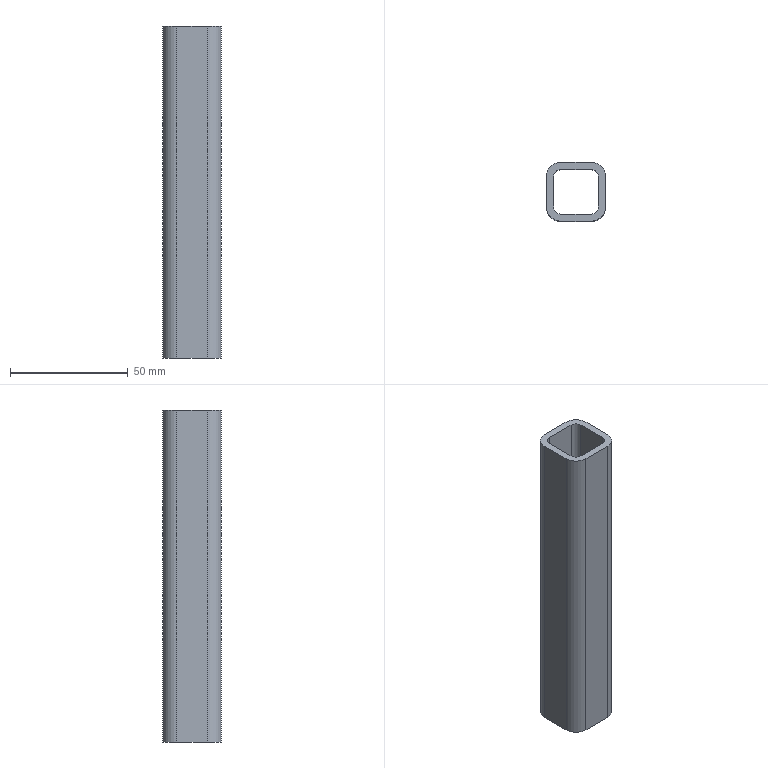Part | STEP file | ISO 10799-2 25x25x3 1784906821283 | 1 solid | 18 faces | box 25 x 25 x 141 mm | volume 33956 mm3 | plane 10 | cylinder 8 | commonest cylinder face diameters 6 x4 12 x4
STEP:
#1=CARTESIAN_POINT('',(-6.5,-9.5,183.));
#2=VERTEX_POINT('',#1);
#3=CARTESIAN_POINT('',(6.5,-9.5,183.));
#4=VERTEX_POINT('',#3);
#5=CARTESIAN_POINT('',(3.25,-9.5,183.));
#6=DIRECTION('',(1.,0.,0.));
#7=VECTOR('',#6,10.);
#8=LINE('',#5,#7);
#9=EDGE_CURVE('',#2,#4,#8,.T.);
#10=ORIENTED_EDGE('',*,*,#9,.T.);
#11=CARTESIAN_POINT('',(6.5,-9.5,41.999));
#12=VERTEX_POINT('',#11);
#13=CARTESIAN_POINT('',(6.5,-9.5,0.));
#14=DIRECTION('',(0.,0.,1.));
#15=VECTOR('',#14,10.);
#16=LINE('',#13,#15);
#17=EDGE_CURVE('',#12,#4,#16,.T.);
#18=ORIENTED_EDGE('',*,*,#17,.F.);
#19=CARTESIAN_POINT('',(-6.5,-9.5,41.999));
#20=VERTEX_POINT('',#19);
#21=CARTESIAN_POINT('',(3.25,-9.5,41.999));
#22=DIRECTION('',(1.,0.,0.));
#23=VECTOR('',#22,10.);
#24=LINE('',#21,#23);
#25=EDGE_CURVE('',#20,#12,#24,.T.);
#26=ORIENTED_EDGE('',*,*,#25,.F.);
#27=CARTESIAN_POINT('',(-6.5,-9.5,0.));
#28=DIRECTION('',(0.,0.,1.));
#29=VECTOR('',#28,10.);
#30=LINE('',#27,#29);
#31=EDGE_CURVE('',#20,#2,#30,.T.);
#32=ORIENTED_EDGE('',*,*,#31,.T.);
#33=EDGE_LOOP('',(#10,#18,#26,#32));
#34=FACE_OUTER_BOUND('',#33,.T.);
#35=CARTESIAN_POINT('',(6.5,-9.5,0.));
#36=DIRECTION('',(0.,-1.,0.));
#37=DIRECTION('',(0.,0.,-1.));
#38=AXIS2_PLACEMENT_3D('',#35,#36,#37);
#39=PLANE('',#38);
#40=ADVANCED_FACE('',(#34),#39,.F.);
#41=CARTESIAN_POINT('',(9.5,-6.5,183.));
#42=VERTEX_POINT('',#41);
#43=CARTESIAN_POINT('',(6.5,-6.5,183.));
#44=DIRECTION('',(0.,0.,1.));
#45=DIRECTION('',(0.,1.,0.));
#46=AXIS2_PLACEMENT_3D('',#43,#44,#45);
#47=CIRCLE('',#46,3.);
#48=EDGE_CURVE('',#4,#42,#47,.T.);
#49=ORIENTED_EDGE('',*,*,#48,.T.);
#50=CARTESIAN_POINT('',(9.5,-6.5,41.999));
#51=VERTEX_POINT('',#50);
#52=CARTESIAN_POINT('',(9.5,-6.5,0.));
#53=DIRECTION('',(0.,0.,1.));
#54=VECTOR('',#53,10.);
#55=LINE('',#52,#54);
#56=EDGE_CURVE('',#51,#42,#55,.T.);
#57=ORIENTED_EDGE('',*,*,#56,.F.);
#58=CARTESIAN_POINT('',(6.5,-6.5,41.999));
#59=DIRECTION('',(0.,0.,1.));
#60=DIRECTION('',(0.,1.,0.));
#61=AXIS2_PLACEMENT_3D('',#58,#59,#60);
#62=CIRCLE('',#61,3.);
#63=EDGE_CURVE('',#12,#51,#62,.T.);
#64=ORIENTED_EDGE('',*,*,#63,.F.);
#65=ORIENTED_EDGE('',*,*,#17,.T.);
#66=EDGE_LOOP('',(#49,#57,#64,#65));
#67=FACE_OUTER_BOUND('',#66,.T.);
#68=CARTESIAN_POINT('',(6.5,-6.5,0.));
#69=DIRECTION('',(0.,0.,1.));
#70=DIRECTION('',(0.,1.,0.));
#71=AXIS2_PLACEMENT_3D('',#68,#69,#70);
#72=CYLINDRICAL_SURFACE('',#71,3.);
#73=ADVANCED_FACE('',(#67),#72,.F.);
#74=CARTESIAN_POINT('',(9.5,6.5,183.));
#75=VERTEX_POINT('',#74);
#76=CARTESIAN_POINT('',(9.5,3.25,183.));
#77=DIRECTION('',(0.,1.,0.));
#78=VECTOR('',#77,10.);
#79=LINE('',#76,#78);
#80=EDGE_CURVE('',#42,#75,#79,.T.);
#81=ORIENTED_EDGE('',*,*,#80,.T.);
#82=CARTESIAN_POINT('',(9.5,6.5,41.999));
#83=VERTEX_POINT('',#82);
#84=CARTESIAN_POINT('',(9.5,6.5,0.));
#85=DIRECTION('',(0.,0.,1.));
#86=VECTOR('',#85,10.);
#87=LINE('',#84,#86);
#88=EDGE_CURVE('',#83,#75,#87,.T.);
#89=ORIENTED_EDGE('',*,*,#88,.F.);
#90=CARTESIAN_POINT('',(9.5,3.25,41.999));
#91=DIRECTION('',(0.,1.,0.));
#92=VECTOR('',#91,10.);
#93=LINE('',#90,#92);
#94=EDGE_CURVE('',#51,#83,#93,.T.);
#95=ORIENTED_EDGE('',*,*,#94,.F.);
#96=ORIENTED_EDGE('',*,*,#56,.T.);
#97=EDGE_LOOP('',(#81,#89,#95,#96));
#98=FACE_OUTER_BOUND('',#97,.T.);
#99=CARTESIAN_POINT('',(9.5,6.5,0.));
#100=DIRECTION('',(1.,0.,0.));
#101=DIRECTION('',(0.,0.,-1.));
#102=AXIS2_PLACEMENT_3D('',#99,#100,#101);
#103=PLANE('',#102);
#104=ADVANCED_FACE('',(#98),#103,.F.);
#105=CARTESIAN_POINT('',(6.5,9.5,183.));
#106=VERTEX_POINT('',#105);
#107=CARTESIAN_POINT('',(6.5,6.5,183.));
#108=DIRECTION('',(0.,0.,1.));
#109=DIRECTION('',(-1.,0.,0.));
#110=AXIS2_PLACEMENT_3D('',#107,#108,#109);
#111=CIRCLE('',#110,3.);
#112=EDGE_CURVE('',#75,#106,#111,.T.);
#113=ORIENTED_EDGE('',*,*,#112,.T.);
#114=CARTESIAN_POINT('',(6.5,9.5,41.999));
#115=VERTEX_POINT('',#114);
#116=CARTESIAN_POINT('',(6.5,9.5,0.));
#117=DIRECTION('',(0.,0.,1.));
#118=VECTOR('',#117,10.);
#119=LINE('',#116,#118);
#120=EDGE_CURVE('',#115,#106,#119,.T.);
#121=ORIENTED_EDGE('',*,*,#120,.F.);
#122=CARTESIAN_POINT('',(6.5,6.5,41.999));
#123=DIRECTION('',(0.,0.,1.));
#124=DIRECTION('',(-1.,0.,0.));
#125=AXIS2_PLACEMENT_3D('',#122,#123,#124);
#126=CIRCLE('',#125,3.);
#127=EDGE_CURVE('',#83,#115,#126,.T.);
#128=ORIENTED_EDGE('',*,*,#127,.F.);
#129=ORIENTED_EDGE('',*,*,#88,.T.);
#130=EDGE_LOOP('',(#113,#121,#128,#129));
#131=FACE_OUTER_BOUND('',#130,.T.);
#132=CARTESIAN_POINT('',(6.5,6.5,0.));
#133=DIRECTION('',(0.,0.,1.));
#134=DIRECTION('',(-1.,0.,0.));
#135=AXIS2_PLACEMENT_3D('',#132,#133,#134);
#136=CYLINDRICAL_SURFACE('',#135,3.);
#137=ADVANCED_FACE('',(#131),#136,.F.);
#138=CARTESIAN_POINT('',(12.5,6.5,183.));
#139=VERTEX_POINT('',#138);
#140=CARTESIAN_POINT('',(12.5,-6.5,183.));
#141=VERTEX_POINT('',#140);
#142=CARTESIAN_POINT('',(12.5,3.25,183.));
#143=DIRECTION('',(0.,-1.,0.));
#144=VECTOR('',#143,10.);
#145=LINE('',#142,#144);
#146=EDGE_CURVE('',#139,#141,#145,.T.);
#147=ORIENTED_EDGE('',*,*,#146,.T.);
#148=CARTESIAN_POINT('',(12.5,-6.5,41.999));
#149=VERTEX_POINT('',#148);
#150=CARTESIAN_POINT('',(12.5,-6.5,0.));
#151=DIRECTION('',(0.,0.,1.));
#152=VECTOR('',#151,10.);
#153=LINE('',#150,#152);
#154=EDGE_CURVE('',#149,#141,#153,.T.);
#155=ORIENTED_EDGE('',*,*,#154,.F.);
#156=CARTESIAN_POINT('',(12.5,6.5,41.999));
#157=VERTEX_POINT('',#156);
#158=CARTESIAN_POINT('',(12.5,3.25,41.999));
#159=DIRECTION('',(0.,-1.,0.));
#160=VECTOR('',#159,10.);
#161=LINE('',#158,#160);
#162=EDGE_CURVE('',#157,#149,#161,.T.);
#163=ORIENTED_EDGE('',*,*,#162,.F.);
#164=CARTESIAN_POINT('',(12.5,6.5,0.));
#165=DIRECTION('',(0.,0.,1.));
#166=VECTOR('',#165,10.);
#167=LINE('',#164,#166);
#168=EDGE_CURVE('',#157,#139,#167,.T.);
#169=ORIENTED_EDGE('',*,*,#168,.T.);
#170=EDGE_LOOP('',(#147,#155,#163,#169));
#171=FACE_OUTER_BOUND('',#170,.T.);
#172=CARTESIAN_POINT('',(12.5,6.5,0.));
#173=DIRECTION('',(1.,0.,0.));
#174=DIRECTION('',(0.,0.,-1.));
#175=AXIS2_PLACEMENT_3D('',#172,#173,#174);
#176=PLANE('',#175);
#177=ADVANCED_FACE('',(#171),#176,.T.);
#178=CARTESIAN_POINT('',(6.5,-12.5,183.));
#179=VERTEX_POINT('',#178);
#180=CARTESIAN_POINT('',(6.5,-6.5,183.));
#181=DIRECTION('',(0.,0.,-1.));
#182=DIRECTION('',(0.,1.,0.));
#183=AXIS2_PLACEMENT_3D('',#180,#181,#182);
#184=CIRCLE('',#183,6.);
#185=EDGE_CURVE('',#141,#179,#184,.T.);
#186=ORIENTED_EDGE('',*,*,#185,.T.);
#187=CARTESIAN_POINT('',(6.5,-12.5,41.999));
#188=VERTEX_POINT('',#187);
#189=CARTESIAN_POINT('',(6.5,-12.5,0.));
#190=DIRECTION('',(0.,0.,1.));
#191=VECTOR('',#190,10.);
#192=LINE('',#189,#191);
#193=EDGE_CURVE('',#188,#179,#192,.T.);
#194=ORIENTED_EDGE('',*,*,#193,.F.);
#195=CARTESIAN_POINT('',(6.5,-6.5,41.999));
#196=DIRECTION('',(0.,0.,-1.));
#197=DIRECTION('',(0.,1.,0.));
#198=AXIS2_PLACEMENT_3D('',#195,#196,#197);
#199=CIRCLE('',#198,6.);
#200=EDGE_CURVE('',#149,#188,#199,.T.);
#201=ORIENTED_EDGE('',*,*,#200,.F.);
#202=ORIENTED_EDGE('',*,*,#154,.T.);
#203=EDGE_LOOP('',(#186,#194,#201,#202));
#204=FACE_OUTER_BOUND('',#203,.T.);
#205=CARTESIAN_POINT('',(6.5,-6.5,0.));
#206=DIRECTION('',(0.,0.,1.));
#207=DIRECTION('',(0.,1.,0.));
#208=AXIS2_PLACEMENT_3D('',#205,#206,#207);
#209=CYLINDRICAL_SURFACE('',#208,6.);
#210=ADVANCED_FACE('',(#204),#209,.T.);
#211=CARTESIAN_POINT('',(-6.5,-12.5,183.));
#212=VERTEX_POINT('',#211);
#213=CARTESIAN_POINT('',(3.25,-12.5,183.));
#214=DIRECTION('',(-1.,0.,0.));
#215=VECTOR('',#214,10.);
#216=LINE('',#213,#215);
#217=EDGE_CURVE('',#179,#212,#216,.T.);
#218=ORIENTED_EDGE('',*,*,#217,.T.);
#219=CARTESIAN_POINT('',(-6.5,-12.5,41.999));
#220=VERTEX_POINT('',#219);
#221=CARTESIAN_POINT('',(-6.5,-12.5,0.));
#222=DIRECTION('',(0.,0.,1.));
#223=VECTOR('',#222,10.);
#224=LINE('',#221,#223);
#225=EDGE_CURVE('',#220,#212,#224,.T.);
#226=ORIENTED_EDGE('',*,*,#225,.F.);
#227=CARTESIAN_POINT('',(3.25,-12.5,41.999));
#228=DIRECTION('',(-1.,0.,0.));
#229=VECTOR('',#228,10.);
#230=LINE('',#227,#229);
#231=EDGE_CURVE('',#188,#220,#230,.T.);
#232=ORIENTED_EDGE('',*,*,#231,.F.);
#233=ORIENTED_EDGE('',*,*,#193,.T.);
#234=EDGE_LOOP('',(#218,#226,#232,#233));
#235=FACE_OUTER_BOUND('',#234,.T.);
#236=CARTESIAN_POINT('',(6.5,-12.5,0.));
#237=DIRECTION('',(0.,-1.,0.));
#238=DIRECTION('',(0.,0.,-1.));
#239=AXIS2_PLACEMENT_3D('',#236,#237,#238);
#240=PLANE('',#239);
#241=ADVANCED_FACE('',(#235),#240,.T.);
#242=CARTESIAN_POINT('',(-12.5,-6.5,183.));
#243=VERTEX_POINT('',#242);
#244=CARTESIAN_POINT('',(-6.5,-6.5,183.));
#245=DIRECTION('',(0.,0.,-1.));
#246=DIRECTION('',(1.,0.,0.));
#247=AXIS2_PLACEMENT_3D('',#244,#245,#246);
#248=CIRCLE('',#247,6.);
#249=EDGE_CURVE('',#212,#243,#248,.T.);
#250=ORIENTED_EDGE('',*,*,#249,.T.);
#251=CARTESIAN_POINT('',(-12.5,-6.5,41.999));
#252=VERTEX_POINT('',#251);
#253=CARTESIAN_POINT('',(-12.5,-6.5,0.));
#254=DIRECTION('',(0.,0.,1.));
#255=VECTOR('',#254,10.);
#256=LINE('',#253,#255);
#257=EDGE_CURVE('',#252,#243,#256,.T.);
#258=ORIENTED_EDGE('',*,*,#257,.F.);
#259=CARTESIAN_POINT('',(-6.5,-6.5,41.999));
#260=DIRECTION('',(0.,0.,-1.));
#261=DIRECTION('',(1.,0.,0.));
#262=AXIS2_PLACEMENT_3D('',#259,#260,#261);
#263=CIRCLE('',#262,6.);
#264=EDGE_CURVE('',#220,#252,#263,.T.);
#265=ORIENTED_EDGE('',*,*,#264,.F.);
#266=ORIENTED_EDGE('',*,*,#225,.T.);
#267=EDGE_LOOP('',(#250,#258,#265,#266));
#268=FACE_OUTER_BOUND('',#267,.T.);
#269=CARTESIAN_POINT('',(-6.5,-6.5,0.));
#270=DIRECTION('',(0.,0.,1.));
#271=DIRECTION('',(1.,0.,0.));
#272=AXIS2_PLACEMENT_3D('',#269,#270,#271);
#273=CYLINDRICAL_SURFACE('',#272,6.);
#274=ADVANCED_FACE('',(#268),#273,.T.);
#275=CARTESIAN_POINT('',(-6.5,9.5,183.));
#276=VERTEX_POINT('',#275);
#277=CARTESIAN_POINT('',(-3.25,9.5,183.));
#278=DIRECTION('',(-1.,0.,0.));
#279=VECTOR('',#278,10.);
#280=LINE('',#277,#279);
#281=EDGE_CURVE('',#106,#276,#280,.T.);
#282=ORIENTED_EDGE('',*,*,#281,.T.);
#283=CARTESIAN_POINT('',(-6.5,9.5,41.999));
#284=VERTEX_POINT('',#283);
#285=CARTESIAN_POINT('',(-6.5,9.5,0.));
#286=DIRECTION('',(0.,0.,1.));
#287=VECTOR('',#286,10.);
#288=LINE('',#285,#287);
#289=EDGE_CURVE('',#284,#276,#288,.T.);
#290=ORIENTED_EDGE('',*,*,#289,.F.);
#291=CARTESIAN_POINT('',(-3.25,9.5,41.999));
#292=DIRECTION('',(-1.,0.,0.));
#293=VECTOR('',#292,10.);
#294=LINE('',#291,#293);
#295=EDGE_CURVE('',#115,#284,#294,.T.);
#296=ORIENTED_EDGE('',*,*,#295,.F.);
#297=ORIENTED_EDGE('',*,*,#120,.T.);
#298=EDGE_LOOP('',(#282,#290,#296,#297));
#299=FACE_OUTER_BOUND('',#298,.T.);
#300=CARTESIAN_POINT('',(-6.5,9.5,0.));
#301=DIRECTION('',(0.,1.,0.));
#302=DIRECTION('',(0.,0.,1.));
#303=AXIS2_PLACEMENT_3D('',#300,#301,#302);
#304=PLANE('',#303);
#305=ADVANCED_FACE('',(#299),#304,.F.);
#306=CARTESIAN_POINT('',(-9.5,-6.5,183.));
#307=VERTEX_POINT('',#306);
#308=CARTESIAN_POINT('',(-6.5,-6.5,183.));
#309=DIRECTION('',(0.,0.,1.));
#310=DIRECTION('',(1.,0.,0.));
#311=AXIS2_PLACEMENT_3D('',#308,#309,#310);
#312=CIRCLE('',#311,3.);
#313=EDGE_CURVE('',#307,#2,#312,.T.);
#314=ORIENTED_EDGE('',*,*,#313,.T.);
#315=ORIENTED_EDGE('',*,*,#31,.F.);
#316=CARTESIAN_POINT('',(-9.5,-6.5,41.999));
#317=VERTEX_POINT('',#316);
#318=CARTESIAN_POINT('',(-6.5,-6.5,41.999));
#319=DIRECTION('',(0.,0.,1.));
#320=DIRECTION('',(1.,0.,0.));
#321=AXIS2_PLACEMENT_3D('',#318,#319,#320);
#322=CIRCLE('',#321,3.);
#323=EDGE_CURVE('',#317,#20,#322,.T.);
#324=ORIENTED_EDGE('',*,*,#323,.F.);
#325=CARTESIAN_POINT('',(-9.5,-6.5,0.));
#326=DIRECTION('',(0.,0.,1.));
#327=VECTOR('',#326,10.);
#328=LINE('',#325,#327);
#329=EDGE_CURVE('',#317,#307,#328,.T.);
#330=ORIENTED_EDGE('',*,*,#329,.T.);
#331=EDGE_LOOP('',(#314,#315,#324,#330));
#332=FACE_OUTER_BOUND('',#331,.T.);
#333=CARTESIAN_POINT('',(-6.5,-6.5,0.));
#334=DIRECTION('',(0.,0.,1.));
#335=DIRECTION('',(1.,0.,0.));
#336=AXIS2_PLACEMENT_3D('',#333,#334,#335);
#337=CYLINDRICAL_SURFACE('',#336,3.);
#338=ADVANCED_FACE('',(#332),#337,.F.);
#339=CARTESIAN_POINT('',(-9.5,6.5,183.));
#340=VERTEX_POINT('',#339);
#341=CARTESIAN_POINT('',(-9.5,-3.25,183.));
#342=DIRECTION('',(0.,-1.,0.));
#343=VECTOR('',#342,10.);
#344=LINE('',#341,#343);
#345=EDGE_CURVE('',#340,#307,#344,.T.);
#346=ORIENTED_EDGE('',*,*,#345,.T.);
#347=ORIENTED_EDGE('',*,*,#329,.F.);
#348=CARTESIAN_POINT('',(-9.5,6.5,41.999));
#349=VERTEX_POINT('',#348);
#350=CARTESIAN_POINT('',(-9.5,-3.25,41.999));
#351=DIRECTION('',(0.,-1.,0.));
#352=VECTOR('',#351,10.);
#353=LINE('',#350,#352);
#354=EDGE_CURVE('',#349,#317,#353,.T.);
#355=ORIENTED_EDGE('',*,*,#354,.F.);
#356=CARTESIAN_POINT('',(-9.5,6.5,0.));
#357=DIRECTION('',(0.,0.,1.));
#358=VECTOR('',#357,10.);
#359=LINE('',#356,#358);
#360=EDGE_CURVE('',#349,#340,#359,.T.);
#361=ORIENTED_EDGE('',*,*,#360,.T.);
#362=EDGE_LOOP('',(#346,#347,#355,#361));
#363=FACE_OUTER_BOUND('',#362,.T.);
#364=CARTESIAN_POINT('',(-9.5,-6.5,0.));
#365=DIRECTION('',(-1.,0.,0.));
#366=DIRECTION('',(0.,0.,1.));
#367=AXIS2_PLACEMENT_3D('',#364,#365,#366);
#368=PLANE('',#367);
#369=ADVANCED_FACE('',(#363),#368,.F.);
#370=CARTESIAN_POINT('',(-6.5,6.5,183.));
#371=DIRECTION('',(0.,0.,1.));
#372=DIRECTION('',(0.,-1.,0.));
#373=AXIS2_PLACEMENT_3D('',#370,#371,#372);
#374=CIRCLE('',#373,3.);
#375=EDGE_CURVE('',#276,#340,#374,.T.);
#376=ORIENTED_EDGE('',*,*,#375,.T.);
#377=ORIENTED_EDGE('',*,*,#360,.F.);
#378=CARTESIAN_POINT('',(-6.5,6.5,41.999));
#379=DIRECTION('',(0.,0.,1.));
#380=DIRECTION('',(0.,-1.,0.));
#381=AXIS2_PLACEMENT_3D('',#378,#379,#380);
#382=CIRCLE('',#381,3.);
#383=EDGE_CURVE('',#284,#349,#382,.T.);
#384=ORIENTED_EDGE('',*,*,#383,.F.);
#385=ORIENTED_EDGE('',*,*,#289,.T.);
#386=EDGE_LOOP('',(#376,#377,#384,#385));
#387=FACE_OUTER_BOUND('',#386,.T.);
#388=CARTESIAN_POINT('',(-6.5,6.5,0.));
#389=DIRECTION('',(0.,0.,1.));
#390=DIRECTION('',(0.,-1.,0.));
#391=AXIS2_PLACEMENT_3D('',#388,#389,#390);
#392=CYLINDRICAL_SURFACE('',#391,3.);
#393=ADVANCED_FACE('',(#387),#392,.F.);
#394=CARTESIAN_POINT('',(-12.5,6.5,183.));
#395=VERTEX_POINT('',#394);
#396=CARTESIAN_POINT('',(-12.5,-3.25,183.));
#397=DIRECTION('',(0.,1.,0.));
#398=VECTOR('',#397,10.);
#399=LINE('',#396,#398);
#400=EDGE_CURVE('',#243,#395,#399,.T.);
#401=ORIENTED_EDGE('',*,*,#400,.T.);
#402=CARTESIAN_POINT('',(-12.5,6.5,41.999));
#403=VERTEX_POINT('',#402);
#404=CARTESIAN_POINT('',(-12.5,6.5,0.));
#405=DIRECTION('',(0.,0.,1.));
#406=VECTOR('',#405,10.);
#407=LINE('',#404,#406);
#408=EDGE_CURVE('',#403,#395,#407,.T.);
#409=ORIENTED_EDGE('',*,*,#408,.F.);
#410=CARTESIAN_POINT('',(-12.5,-3.25,41.999));
#411=DIRECTION('',(0.,1.,0.));
#412=VECTOR('',#411,10.);
#413=LINE('',#410,#412);
#414=EDGE_CURVE('',#252,#403,#413,.T.);
#415=ORIENTED_EDGE('',*,*,#414,.F.);
#416=ORIENTED_EDGE('',*,*,#257,.T.);
#417=EDGE_LOOP('',(#401,#409,#415,#416));
#418=FACE_OUTER_BOUND('',#417,.T.);
#419=CARTESIAN_POINT('',(-12.5,-6.5,0.));
#420=DIRECTION('',(-1.,0.,0.));
#421=DIRECTION('',(0.,0.,1.));
#422=AXIS2_PLACEMENT_3D('',#419,#420,#421);
#423=PLANE('',#422);
#424=ADVANCED_FACE('',(#418),#423,.T.);
#425=CARTESIAN_POINT('',(-6.5,12.5,183.));
#426=VERTEX_POINT('',#425);
#427=CARTESIAN_POINT('',(-6.5,6.5,183.));
#428=DIRECTION('',(0.,0.,-1.));
#429=DIRECTION('',(0.,-1.,0.));
#430=AXIS2_PLACEMENT_3D('',#427,#428,#429);
#431=CIRCLE('',#430,6.);
#432=EDGE_CURVE('',#395,#426,#431,.T.);
#433=ORIENTED_EDGE('',*,*,#432,.T.);
#434=CARTESIAN_POINT('',(-6.5,12.5,41.999));
#435=VERTEX_POINT('',#434);
#436=CARTESIAN_POINT('',(-6.5,12.5,0.));
#437=DIRECTION('',(0.,0.,1.));
#438=VECTOR('',#437,10.);
#439=LINE('',#436,#438);
#440=EDGE_CURVE('',#435,#426,#439,.T.);
#441=ORIENTED_EDGE('',*,*,#440,.F.);
#442=CARTESIAN_POINT('',(-6.5,6.5,41.999));
#443=DIRECTION('',(0.,0.,-1.));
#444=DIRECTION('',(0.,-1.,0.));
#445=AXIS2_PLACEMENT_3D('',#442,#443,#444);
#446=CIRCLE('',#445,6.);
#447=EDGE_CURVE('',#403,#435,#446,.T.);
#448=ORIENTED_EDGE('',*,*,#447,.F.);
#449=ORIENTED_EDGE('',*,*,#408,.T.);
#450=EDGE_LOOP('',(#433,#441,#448,#449));
#451=FACE_OUTER_BOUND('',#450,.T.);
#452=CARTESIAN_POINT('',(-6.5,6.5,0.));
#453=DIRECTION('',(0.,0.,1.));
#454=DIRECTION('',(0.,-1.,0.));
#455=AXIS2_PLACEMENT_3D('',#452,#453,#454);
#456=CYLINDRICAL_SURFACE('',#455,6.);
#457=ADVANCED_FACE('',(#451),#456,.T.);
#458=CARTESIAN_POINT('',(6.5,12.5,183.));
#459=VERTEX_POINT('',#458);
#460=CARTESIAN_POINT('',(-3.25,12.5,183.));
#461=DIRECTION('',(1.,0.,0.));
#462=VECTOR('',#461,10.);
#463=LINE('',#460,#462);
#464=EDGE_CURVE('',#426,#459,#463,.T.);
#465=ORIENTED_EDGE('',*,*,#464,.T.);
#466=CARTESIAN_POINT('',(6.5,12.5,41.999));
#467=VERTEX_POINT('',#466);
#468=CARTESIAN_POINT('',(6.5,12.5,0.));
#469=DIRECTION('',(0.,0.,1.));
#470=VECTOR('',#469,10.);
#471=LINE('',#468,#470);
#472=EDGE_CURVE('',#467,#459,#471,.T.);
#473=ORIENTED_EDGE('',*,*,#472,.F.);
#474=CARTESIAN_POINT('',(-3.25,12.5,41.999));
#475=DIRECTION('',(1.,0.,0.));
#476=VECTOR('',#475,10.);
#477=LINE('',#474,#476);
#478=EDGE_CURVE('',#435,#467,#477,.T.);
#479=ORIENTED_EDGE('',*,*,#478,.F.);
#480=ORIENTED_EDGE('',*,*,#440,.T.);
#481=EDGE_LOOP('',(#465,#473,#479,#480));
#482=FACE_OUTER_BOUND('',#481,.T.);
#483=CARTESIAN_POINT('',(-6.5,12.5,0.));
#484=DIRECTION('',(0.,1.,0.));
#485=DIRECTION('',(0.,0.,1.));
#486=AXIS2_PLACEMENT_3D('',#483,#484,#485);
#487=PLANE('',#486);
#488=ADVANCED_FACE('',(#482),#487,.T.);
#489=CARTESIAN_POINT('',(6.5,6.5,183.));
#490=DIRECTION('',(0.,0.,-1.));
#491=DIRECTION('',(-1.,0.,0.));
#492=AXIS2_PLACEMENT_3D('',#489,#490,#491);
#493=CIRCLE('',#492,6.);
#494=EDGE_CURVE('',#459,#139,#493,.T.);
#495=ORIENTED_EDGE('',*,*,#494,.T.);
#496=ORIENTED_EDGE('',*,*,#168,.F.);
#497=CARTESIAN_POINT('',(6.5,6.5,41.999));
#498=DIRECTION('',(0.,0.,-1.));
#499=DIRECTION('',(-1.,0.,0.));
#500=AXIS2_PLACEMENT_3D('',#497,#498,#499);
#501=CIRCLE('',#500,6.);
#502=EDGE_CURVE('',#467,#157,#501,.T.);
#503=ORIENTED_EDGE('',*,*,#502,.F.);
#504=ORIENTED_EDGE('',*,*,#472,.T.);
#505=EDGE_LOOP('',(#495,#496,#503,#504));
#506=FACE_OUTER_BOUND('',#505,.T.);
#507=CARTESIAN_POINT('',(6.5,6.5,0.));
#508=DIRECTION('',(0.,0.,1.));
#509=DIRECTION('',(-1.,0.,0.));
#510=AXIS2_PLACEMENT_3D('',#507,#508,#509);
#511=CYLINDRICAL_SURFACE('',#510,6.);
#512=ADVANCED_FACE('',(#506),#511,.T.);
#513=ORIENTED_EDGE('',*,*,#414,.T.);
#514=ORIENTED_EDGE('',*,*,#447,.T.);
#515=ORIENTED_EDGE('',*,*,#478,.T.);
#516=ORIENTED_EDGE('',*,*,#502,.T.);
#517=ORIENTED_EDGE('',*,*,#162,.T.);
#518=ORIENTED_EDGE('',*,*,#200,.T.);
#519=ORIENTED_EDGE('',*,*,#231,.T.);
#520=ORIENTED_EDGE('',*,*,#264,.T.);
#521=EDGE_LOOP('',(#513,#514,#515,#516,#517,#518,#519,#520));
#522=FACE_OUTER_BOUND('',#521,.T.);
#523=ORIENTED_EDGE('',*,*,#295,.T.);
#524=ORIENTED_EDGE('',*,*,#383,.T.);
#525=ORIENTED_EDGE('',*,*,#354,.T.);
#526=ORIENTED_EDGE('',*,*,#323,.T.);
#527=ORIENTED_EDGE('',*,*,#25,.T.);
#528=ORIENTED_EDGE('',*,*,#63,.T.);
#529=ORIENTED_EDGE('',*,*,#94,.T.);
#530=ORIENTED_EDGE('',*,*,#127,.T.);
#531=EDGE_LOOP('',(#523,#524,#525,#526,#527,#528,#529,#530));
#532=FACE_BOUND('',#531,.T.);
#533=CARTESIAN_POINT('',(0.,0.,41.999));
#534=DIRECTION('',(0.,0.,1.));
#535=DIRECTION('',(1.,0.,0.));
#536=AXIS2_PLACEMENT_3D('',#533,#534,#535);
#537=PLANE('',#536);
#538=ADVANCED_FACE('',(#522,#532),#537,.F.);
#539=ORIENTED_EDGE('',*,*,#400,.F.);
#540=ORIENTED_EDGE('',*,*,#249,.F.);
#541=ORIENTED_EDGE('',*,*,#217,.F.);
#542=ORIENTED_EDGE('',*,*,#185,.F.);
#543=ORIENTED_EDGE('',*,*,#146,.F.);
#544=ORIENTED_EDGE('',*,*,#494,.F.);
#545=ORIENTED_EDGE('',*,*,#464,.F.);
#546=ORIENTED_EDGE('',*,*,#432,.F.);
#547=EDGE_LOOP('',(#539,#540,#541,#542,#543,#544,#545,#546));
#548=FACE_OUTER_BOUND('',#547,.T.);
#549=ORIENTED_EDGE('',*,*,#281,.F.);
#550=ORIENTED_EDGE('',*,*,#112,.F.);
#551=ORIENTED_EDGE('',*,*,#80,.F.);
#552=ORIENTED_EDGE('',*,*,#48,.F.);
#553=ORIENTED_EDGE('',*,*,#9,.F.);
#554=ORIENTED_EDGE('',*,*,#313,.F.);
#555=ORIENTED_EDGE('',*,*,#345,.F.);
#556=ORIENTED_EDGE('',*,*,#375,.F.);
#557=EDGE_LOOP('',(#549,#550,#551,#552,#553,#554,#555,#556));
#558=FACE_BOUND('',#557,.T.);
#559=CARTESIAN_POINT('',(0.,0.,183.));
#560=DIRECTION('',(0.,0.,1.));
#561=DIRECTION('',(1.,0.,0.));
#562=AXIS2_PLACEMENT_3D('',#559,#560,#561);
#563=PLANE('',#562);
#564=ADVANCED_FACE('',(#548,#558),#563,.T.);
#565=CLOSED_SHELL('',(#40,#73,#104,#137,#177,#210,#241,#274,#305,#338,#369,#393,#424,#457,#488,#512,#538,#564));
#566=MANIFOLD_SOLID_BREP('',#565);
#567=(LENGTH_UNIT()NAMED_UNIT(*)SI_UNIT(.MILLI.,.METRE.));
#568=UNCERTAINTY_MEASURE_WITH_UNIT(LENGTH_MEASURE(0.01),#567,'','');
#569=(NAMED_UNIT(*)PLANE_ANGLE_UNIT()SI_UNIT($,.RADIAN.));
#570=(NAMED_UNIT(*)SI_UNIT($,.STERADIAN.)SOLID_ANGLE_UNIT());
#571=(GEOMETRIC_REPRESENTATION_CONTEXT(3)GLOBAL_UNCERTAINTY_ASSIGNED_CONTEXT((#568))GLOBAL_UNIT_ASSIGNED_CONTEXT((#567,#569,#570))REPRESENTATION_CONTEXT('',''));
#572=ADVANCED_BREP_SHAPE_REPRESENTATION('',(#566),#571);